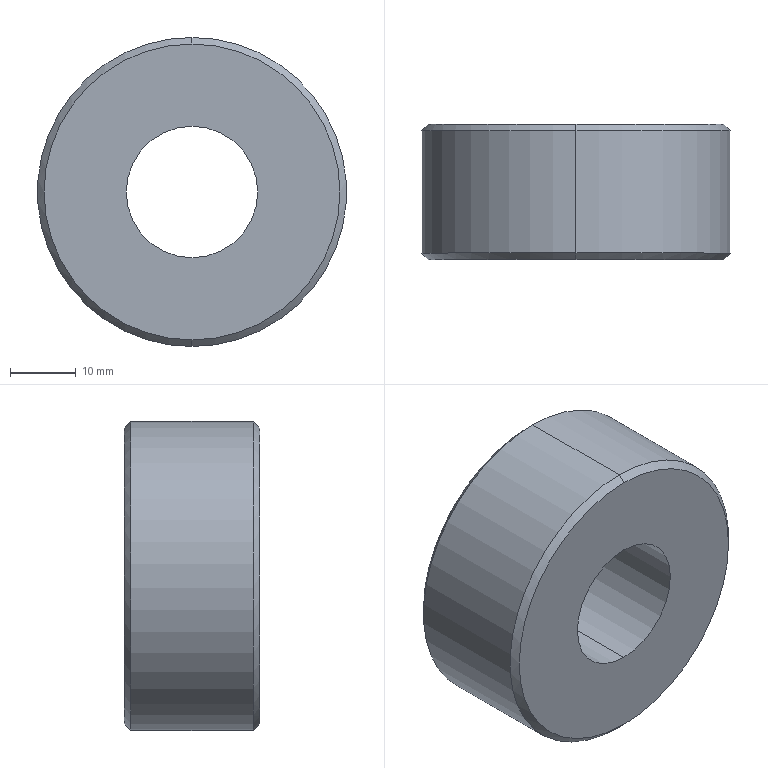Part | SolidWorks | features BaseBody 1 | 1 solid | 10 faces | box 47 x 20.6 x 47 mm | volume 29123 mm3 | cone 4 | cylinder 4 | plane 2 | commonest cylinder face diameters 20 x2 47 x2
STEP:
#1=CARTESIAN_POINT('',(-530.322,-67.,-4.209));
#2=VERTEX_POINT('',#1);
#3=CARTESIAN_POINT('',(-530.322,-67.,40.791));
#4=VERTEX_POINT('',#3);
#5=CARTESIAN_POINT('',(-530.322,-67.,18.291));
#6=DIRECTION('',(0.,1.,0.));
#7=DIRECTION('',(0.,0.,1.));
#8=AXIS2_PLACEMENT_3D('',#5,#6,#7);
#9=CIRCLE('',#8,22.5);
#10=EDGE_CURVE('',#2,#4,#9,.T.);
#11=ORIENTED_EDGE('',*,*,#10,.F.);
#12=CARTESIAN_POINT('',(-530.322,-68.,-5.209));
#13=VERTEX_POINT('',#12);
#14=CARTESIAN_POINT('',(-530.322,-67.,-4.209));
#15=DIRECTION('',(0.,-0.7071,-0.7071));
#16=VECTOR('',#15,1000.);
#17=LINE('',#14,#16);
#18=EDGE_CURVE('',#2,#13,#17,.T.);
#19=ORIENTED_EDGE('',*,*,#18,.T.);
#20=CARTESIAN_POINT('',(-530.322,-68.,41.791));
#21=VERTEX_POINT('',#20);
#22=CARTESIAN_POINT('',(-530.322,-68.,18.291));
#23=DIRECTION('',(0.,-1.,0.));
#24=DIRECTION('',(0.,0.,-1.));
#25=AXIS2_PLACEMENT_3D('',#22,#23,#24);
#26=CIRCLE('',#25,23.5);
#27=EDGE_CURVE('',#21,#13,#26,.T.);
#28=ORIENTED_EDGE('',*,*,#27,.F.);
#29=CARTESIAN_POINT('',(-530.322,-67.,40.791));
#30=DIRECTION('',(0.,-0.7071,0.7071));
#31=VECTOR('',#30,1000.);
#32=LINE('',#29,#31);
#33=EDGE_CURVE('',#4,#21,#32,.T.);
#34=ORIENTED_EDGE('',*,*,#33,.F.);
#35=EDGE_LOOP('',(#11,#19,#28,#34));
#36=FACE_OUTER_BOUND('',#35,.T.);
#37=CARTESIAN_POINT('',(-530.322,-67.,18.291));
#38=DIRECTION('',(0.,-1.,0.));
#39=DIRECTION('',(0.,0.,1.));
#40=AXIS2_PLACEMENT_3D('',#37,#38,#39);
#41=CONICAL_SURFACE('',#40,22.5,0.7854);
#42=ADVANCED_FACE('',(#36),#41,.T.);
#43=CARTESIAN_POINT('',(-530.322,-87.6,40.791));
#44=VERTEX_POINT('',#43);
#45=CARTESIAN_POINT('',(-530.322,-87.6,-4.209));
#46=VERTEX_POINT('',#45);
#47=CARTESIAN_POINT('',(-530.322,-87.6,18.291));
#48=DIRECTION('',(0.,-1.,0.));
#49=DIRECTION('',(0.,0.,1.));
#50=AXIS2_PLACEMENT_3D('',#47,#48,#49);
#51=CIRCLE('',#50,22.5);
#52=EDGE_CURVE('',#44,#46,#51,.T.);
#53=ORIENTED_EDGE('',*,*,#52,.F.);
#54=CARTESIAN_POINT('',(-530.322,-86.6,41.791));
#55=VERTEX_POINT('',#54);
#56=CARTESIAN_POINT('',(-530.322,-86.6,41.791));
#57=DIRECTION('',(0.,0.7071,0.7071));
#58=VECTOR('',#57,1000.);
#59=LINE('',#56,#58);
#60=EDGE_CURVE('',#44,#55,#59,.T.);
#61=ORIENTED_EDGE('',*,*,#60,.T.);
#62=CARTESIAN_POINT('',(-530.322,-86.6,-5.209));
#63=VERTEX_POINT('',#62);
#64=CARTESIAN_POINT('',(-530.322,-86.6,18.291));
#65=DIRECTION('',(0.,1.,0.));
#66=DIRECTION('',(0.,0.,1.));
#67=AXIS2_PLACEMENT_3D('',#64,#65,#66);
#68=CIRCLE('',#67,23.5);
#69=EDGE_CURVE('',#63,#55,#68,.T.);
#70=ORIENTED_EDGE('',*,*,#69,.F.);
#71=CARTESIAN_POINT('',(-530.322,-86.6,-5.209));
#72=DIRECTION('',(0.,0.7071,-0.7071));
#73=VECTOR('',#72,1000.);
#74=LINE('',#71,#73);
#75=EDGE_CURVE('',#46,#63,#74,.T.);
#76=ORIENTED_EDGE('',*,*,#75,.F.);
#77=EDGE_LOOP('',(#53,#61,#70,#76));
#78=FACE_OUTER_BOUND('',#77,.T.);
#79=CARTESIAN_POINT('',(-530.322,-86.6,18.291));
#80=DIRECTION('',(0.,1.,0.));
#81=DIRECTION('',(0.,0.,-1.));
#82=AXIS2_PLACEMENT_3D('',#79,#80,#81);
#83=CONICAL_SURFACE('',#82,23.5,0.7854);
#84=ADVANCED_FACE('',(#78),#83,.T.);
#85=ORIENTED_EDGE('',*,*,#69,.T.);
#86=CARTESIAN_POINT('',(-530.322,-87.6,41.791));
#87=DIRECTION('',(0.,1.,0.));
#88=VECTOR('',#87,1000.);
#89=LINE('',#86,#88);
#90=EDGE_CURVE('',#55,#21,#89,.T.);
#91=ORIENTED_EDGE('',*,*,#90,.T.);
#92=ORIENTED_EDGE('',*,*,#27,.T.);
#93=CARTESIAN_POINT('',(-530.322,-87.6,-5.209));
#94=DIRECTION('',(0.,1.,0.));
#95=VECTOR('',#94,1000.);
#96=LINE('',#93,#95);
#97=EDGE_CURVE('',#63,#13,#96,.T.);
#98=ORIENTED_EDGE('',*,*,#97,.F.);
#99=EDGE_LOOP('',(#85,#91,#92,#98));
#100=FACE_OUTER_BOUND('',#99,.T.);
#101=CARTESIAN_POINT('',(-530.322,-87.6,18.291));
#102=DIRECTION('',(0.,1.,0.));
#103=DIRECTION('',(0.,0.,-1.));
#104=AXIS2_PLACEMENT_3D('',#101,#102,#103);
#105=CYLINDRICAL_SURFACE('',#104,23.5);
#106=ADVANCED_FACE('',(#100),#105,.T.);
#107=CARTESIAN_POINT('',(-530.322,-87.6,8.291));
#108=VERTEX_POINT('',#107);
#109=CARTESIAN_POINT('',(-530.322,-87.6,28.291));
#110=VERTEX_POINT('',#109);
#111=CARTESIAN_POINT('',(-530.322,-87.6,18.291));
#112=DIRECTION('',(0.,-1.,0.));
#113=DIRECTION('',(0.,0.,1.));
#114=AXIS2_PLACEMENT_3D('',#111,#112,#113);
#115=CIRCLE('',#114,10.);
#116=EDGE_CURVE('',#108,#110,#115,.T.);
#117=ORIENTED_EDGE('',*,*,#116,.T.);
#118=CARTESIAN_POINT('',(-530.322,-67.,28.291));
#119=VERTEX_POINT('',#118);
#120=CARTESIAN_POINT('',(-530.322,-87.6,28.291));
#121=DIRECTION('',(0.,1.,0.));
#122=VECTOR('',#121,1000.);
#123=LINE('',#120,#122);
#124=EDGE_CURVE('',#110,#119,#123,.T.);
#125=ORIENTED_EDGE('',*,*,#124,.T.);
#126=CARTESIAN_POINT('',(-530.322,-67.,8.291));
#127=VERTEX_POINT('',#126);
#128=CARTESIAN_POINT('',(-530.322,-67.,18.291));
#129=DIRECTION('',(0.,-1.,0.));
#130=DIRECTION('',(0.,0.,1.));
#131=AXIS2_PLACEMENT_3D('',#128,#129,#130);
#132=CIRCLE('',#131,10.);
#133=EDGE_CURVE('',#127,#119,#132,.T.);
#134=ORIENTED_EDGE('',*,*,#133,.F.);
#135=CARTESIAN_POINT('',(-530.322,-87.6,8.291));
#136=DIRECTION('',(0.,1.,0.));
#137=VECTOR('',#136,1000.);
#138=LINE('',#135,#137);
#139=EDGE_CURVE('',#108,#127,#138,.T.);
#140=ORIENTED_EDGE('',*,*,#139,.F.);
#141=EDGE_LOOP('',(#117,#125,#134,#140));
#142=FACE_OUTER_BOUND('',#141,.T.);
#143=CARTESIAN_POINT('',(-530.322,-87.6,18.291));
#144=DIRECTION('',(0.,1.,0.));
#145=DIRECTION('',(0.,0.,-1.));
#146=AXIS2_PLACEMENT_3D('',#143,#144,#145);
#147=CYLINDRICAL_SURFACE('',#146,10.);
#148=ADVANCED_FACE('',(#142),#147,.F.);
#149=ORIENTED_EDGE('',*,*,#133,.T.);
#150=CARTESIAN_POINT('',(-530.322,-67.,18.291));
#151=DIRECTION('',(0.,-1.,0.));
#152=DIRECTION('',(0.,0.,1.));
#153=AXIS2_PLACEMENT_3D('',#150,#151,#152);
#154=CIRCLE('',#153,10.);
#155=EDGE_CURVE('',#119,#127,#154,.T.);
#156=ORIENTED_EDGE('',*,*,#155,.T.);
#157=EDGE_LOOP('',(#149,#156));
#158=FACE_BOUND('',#157,.T.);
#159=CARTESIAN_POINT('',(-530.322,-67.,18.291));
#160=DIRECTION('',(0.,1.,0.));
#161=DIRECTION('',(0.,0.,1.));
#162=AXIS2_PLACEMENT_3D('',#159,#160,#161);
#163=CIRCLE('',#162,22.5);
#164=EDGE_CURVE('',#4,#2,#163,.T.);
#165=ORIENTED_EDGE('',*,*,#164,.T.);
#166=ORIENTED_EDGE('',*,*,#10,.T.);
#167=EDGE_LOOP('',(#165,#166));
#168=FACE_OUTER_BOUND('',#167,.T.);
#169=CARTESIAN_POINT('',(-530.322,-67.,18.291));
#170=DIRECTION('',(0.,1.,0.));
#171=DIRECTION('',(1.,0.,0.));
#172=AXIS2_PLACEMENT_3D('',#169,#170,#171);
#173=PLANE('',#172);
#174=ADVANCED_FACE('',(#158,#168),#173,.T.);
#175=ORIENTED_EDGE('',*,*,#116,.F.);
#176=CARTESIAN_POINT('',(-530.322,-87.6,18.291));
#177=DIRECTION('',(0.,-1.,0.));
#178=DIRECTION('',(0.,0.,1.));
#179=AXIS2_PLACEMENT_3D('',#176,#177,#178);
#180=CIRCLE('',#179,10.);
#181=EDGE_CURVE('',#110,#108,#180,.T.);
#182=ORIENTED_EDGE('',*,*,#181,.F.);
#183=EDGE_LOOP('',(#175,#182));
#184=FACE_BOUND('',#183,.T.);
#185=CARTESIAN_POINT('',(-530.322,-87.6,18.291));
#186=DIRECTION('',(0.,-1.,0.));
#187=DIRECTION('',(0.,0.,1.));
#188=AXIS2_PLACEMENT_3D('',#185,#186,#187);
#189=CIRCLE('',#188,22.5);
#190=EDGE_CURVE('',#46,#44,#189,.T.);
#191=ORIENTED_EDGE('',*,*,#190,.T.);
#192=ORIENTED_EDGE('',*,*,#52,.T.);
#193=EDGE_LOOP('',(#191,#192));
#194=FACE_OUTER_BOUND('',#193,.T.);
#195=CARTESIAN_POINT('',(-530.322,-87.6,18.291));
#196=DIRECTION('',(0.,1.,0.));
#197=DIRECTION('',(1.,0.,0.));
#198=AXIS2_PLACEMENT_3D('',#195,#196,#197);
#199=PLANE('',#198);
#200=ADVANCED_FACE('',(#184,#194),#199,.F.);
#201=ORIENTED_EDGE('',*,*,#124,.F.);
#202=ORIENTED_EDGE('',*,*,#181,.T.);
#203=ORIENTED_EDGE('',*,*,#139,.T.);
#204=ORIENTED_EDGE('',*,*,#155,.F.);
#205=EDGE_LOOP('',(#201,#202,#203,#204));
#206=FACE_OUTER_BOUND('',#205,.T.);
#207=CARTESIAN_POINT('',(-530.322,-87.6,18.291));
#208=DIRECTION('',(0.,1.,0.));
#209=DIRECTION('',(0.,0.,-1.));
#210=AXIS2_PLACEMENT_3D('',#207,#208,#209);
#211=CYLINDRICAL_SURFACE('',#210,10.);
#212=ADVANCED_FACE('',(#206),#211,.F.);
#213=ORIENTED_EDGE('',*,*,#90,.F.);
#214=CARTESIAN_POINT('',(-530.322,-86.6,18.291));
#215=DIRECTION('',(0.,1.,0.));
#216=DIRECTION('',(0.,0.,1.));
#217=AXIS2_PLACEMENT_3D('',#214,#215,#216);
#218=CIRCLE('',#217,23.5);
#219=EDGE_CURVE('',#55,#63,#218,.T.);
#220=ORIENTED_EDGE('',*,*,#219,.T.);
#221=ORIENTED_EDGE('',*,*,#97,.T.);
#222=CARTESIAN_POINT('',(-530.322,-68.,18.291));
#223=DIRECTION('',(0.,-1.,0.));
#224=DIRECTION('',(0.,0.,-1.));
#225=AXIS2_PLACEMENT_3D('',#222,#223,#224);
#226=CIRCLE('',#225,23.5);
#227=EDGE_CURVE('',#13,#21,#226,.T.);
#228=ORIENTED_EDGE('',*,*,#227,.T.);
#229=EDGE_LOOP('',(#213,#220,#221,#228));
#230=FACE_OUTER_BOUND('',#229,.T.);
#231=CARTESIAN_POINT('',(-530.322,-87.6,18.291));
#232=DIRECTION('',(0.,1.,0.));
#233=DIRECTION('',(0.,0.,-1.));
#234=AXIS2_PLACEMENT_3D('',#231,#232,#233);
#235=CYLINDRICAL_SURFACE('',#234,23.5);
#236=ADVANCED_FACE('',(#230),#235,.T.);
#237=ORIENTED_EDGE('',*,*,#60,.F.);
#238=ORIENTED_EDGE('',*,*,#190,.F.);
#239=ORIENTED_EDGE('',*,*,#75,.T.);
#240=ORIENTED_EDGE('',*,*,#219,.F.);
#241=EDGE_LOOP('',(#237,#238,#239,#240));
#242=FACE_OUTER_BOUND('',#241,.T.);
#243=CARTESIAN_POINT('',(-530.322,-86.6,18.291));
#244=DIRECTION('',(0.,1.,0.));
#245=DIRECTION('',(0.,0.,-1.));
#246=AXIS2_PLACEMENT_3D('',#243,#244,#245);
#247=CONICAL_SURFACE('',#246,23.5,0.7854);
#248=ADVANCED_FACE('',(#242),#247,.T.);
#249=ORIENTED_EDGE('',*,*,#18,.F.);
#250=ORIENTED_EDGE('',*,*,#164,.F.);
#251=ORIENTED_EDGE('',*,*,#33,.T.);
#252=ORIENTED_EDGE('',*,*,#227,.F.);
#253=EDGE_LOOP('',(#249,#250,#251,#252));
#254=FACE_OUTER_BOUND('',#253,.T.);
#255=CARTESIAN_POINT('',(-530.322,-67.,18.291));
#256=DIRECTION('',(0.,-1.,0.));
#257=DIRECTION('',(0.,0.,1.));
#258=AXIS2_PLACEMENT_3D('',#255,#256,#257);
#259=CONICAL_SURFACE('',#258,22.5,0.7854);
#260=ADVANCED_FACE('',(#254),#259,.T.);
#261=CLOSED_SHELL('',(#42,#84,#106,#148,#174,#200,#212,#236,#248,#260));
#262=MANIFOLD_SOLID_BREP('',#261);
#263=CARTESIAN_POINT('',(0.,0.,0.));
#264=DIRECTION('',(0.,0.,1.));
#265=DIRECTION('',(1.,0.,0.));
#266=AXIS2_PLACEMENT_3D('',#263,#264,#265);
#267=(LENGTH_UNIT()NAMED_UNIT(*)SI_UNIT(.MILLI.,.METRE.));
#268=UNCERTAINTY_MEASURE_WITH_UNIT(LENGTH_MEASURE(0.00001),#267,'','');
#269=(NAMED_UNIT(*)PLANE_ANGLE_UNIT()SI_UNIT($,.RADIAN.));
#270=(NAMED_UNIT(*)SI_UNIT($,.STERADIAN.)SOLID_ANGLE_UNIT());
#271=(GEOMETRIC_REPRESENTATION_CONTEXT(3)GLOBAL_UNCERTAINTY_ASSIGNED_CONTEXT((#268))GLOBAL_UNIT_ASSIGNED_CONTEXT((#267,#269,#270))REPRESENTATION_CONTEXT('',''));
#272=ADVANCED_BREP_SHAPE_REPRESENTATION('',(#262,#266),#271);